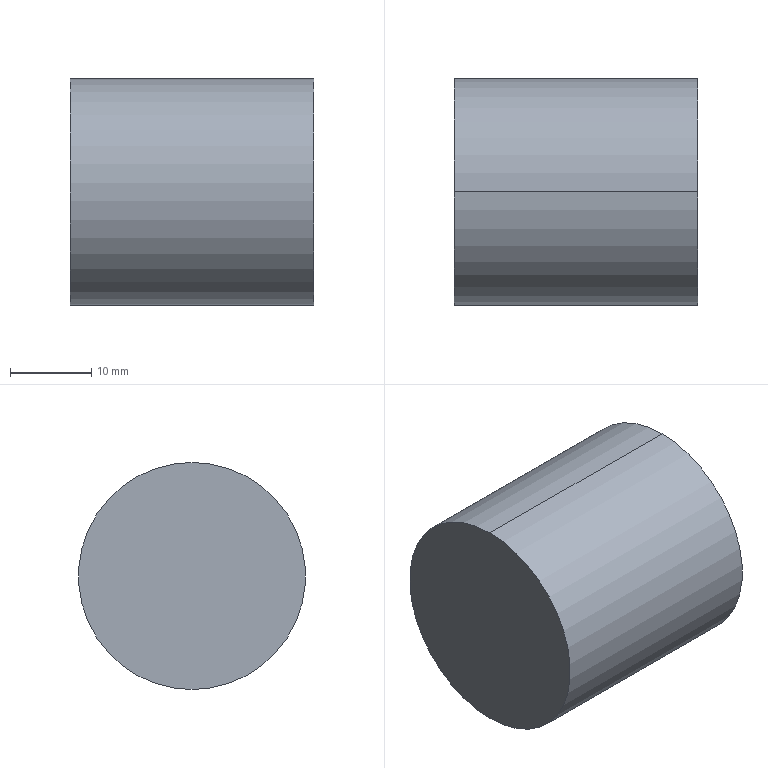Part | SolidWorks | features BaseBody 1 | 1 solid | 4 faces | box 30 x 28 x 28 mm | volume 18473 mm3 | cylinder 2 | plane 2 | commonest cylinder face diameters 28 x2
STEP:
#1=CARTESIAN_POINT('',(104.,23.,-152.));
#2=VERTEX_POINT('',#1);
#3=CARTESIAN_POINT('',(104.,23.,-124.));
#4=VERTEX_POINT('',#3);
#5=CARTESIAN_POINT('',(104.,23.,-138.));
#6=DIRECTION('',(1.,0.,0.));
#7=DIRECTION('',(0.,0.,-1.));
#8=AXIS2_PLACEMENT_3D('',#5,#6,#7);
#9=CIRCLE('',#8,14.);
#10=EDGE_CURVE('',#2,#4,#9,.T.);
#11=ORIENTED_EDGE('',*,*,#10,.T.);
#12=CARTESIAN_POINT('',(134.,23.,-124.));
#13=VERTEX_POINT('',#12);
#14=CARTESIAN_POINT('',(104.,23.,-124.));
#15=DIRECTION('',(1.,0.,0.));
#16=VECTOR('',#15,1000.);
#17=LINE('',#14,#16);
#18=EDGE_CURVE('',#4,#13,#17,.T.);
#19=ORIENTED_EDGE('',*,*,#18,.T.);
#20=CARTESIAN_POINT('',(134.,23.,-152.));
#21=VERTEX_POINT('',#20);
#22=CARTESIAN_POINT('',(134.,23.,-138.));
#23=DIRECTION('',(-1.,0.,0.));
#24=DIRECTION('',(0.,0.,-1.));
#25=AXIS2_PLACEMENT_3D('',#22,#23,#24);
#26=CIRCLE('',#25,14.);
#27=EDGE_CURVE('',#13,#21,#26,.T.);
#28=ORIENTED_EDGE('',*,*,#27,.T.);
#29=CARTESIAN_POINT('',(104.,23.,-152.));
#30=DIRECTION('',(1.,0.,0.));
#31=VECTOR('',#30,1000.);
#32=LINE('',#29,#31);
#33=EDGE_CURVE('',#2,#21,#32,.T.);
#34=ORIENTED_EDGE('',*,*,#33,.F.);
#35=EDGE_LOOP('',(#11,#19,#28,#34));
#36=FACE_OUTER_BOUND('',#35,.T.);
#37=CARTESIAN_POINT('',(104.,23.,-138.));
#38=DIRECTION('',(1.,0.,0.));
#39=DIRECTION('',(0.,0.,-1.));
#40=AXIS2_PLACEMENT_3D('',#37,#38,#39);
#41=CYLINDRICAL_SURFACE('',#40,14.);
#42=ADVANCED_FACE('',(#36),#41,.T.);
#43=ORIENTED_EDGE('',*,*,#18,.F.);
#44=CARTESIAN_POINT('',(104.,23.,-138.));
#45=DIRECTION('',(1.,0.,0.));
#46=DIRECTION('',(0.,0.,-1.));
#47=AXIS2_PLACEMENT_3D('',#44,#45,#46);
#48=CIRCLE('',#47,14.);
#49=EDGE_CURVE('',#4,#2,#48,.T.);
#50=ORIENTED_EDGE('',*,*,#49,.T.);
#51=ORIENTED_EDGE('',*,*,#33,.T.);
#52=CARTESIAN_POINT('',(134.,23.,-138.));
#53=DIRECTION('',(-1.,0.,0.));
#54=DIRECTION('',(0.,0.,-1.));
#55=AXIS2_PLACEMENT_3D('',#52,#53,#54);
#56=CIRCLE('',#55,14.);
#57=EDGE_CURVE('',#21,#13,#56,.T.);
#58=ORIENTED_EDGE('',*,*,#57,.T.);
#59=EDGE_LOOP('',(#43,#50,#51,#58));
#60=FACE_OUTER_BOUND('',#59,.T.);
#61=CARTESIAN_POINT('',(104.,23.,-138.));
#62=DIRECTION('',(1.,0.,0.));
#63=DIRECTION('',(0.,0.,-1.));
#64=AXIS2_PLACEMENT_3D('',#61,#62,#63);
#65=CYLINDRICAL_SURFACE('',#64,14.);
#66=ADVANCED_FACE('',(#60),#65,.T.);
#67=ORIENTED_EDGE('',*,*,#10,.F.);
#68=ORIENTED_EDGE('',*,*,#49,.F.);
#69=EDGE_LOOP('',(#67,#68));
#70=FACE_OUTER_BOUND('',#69,.T.);
#71=CARTESIAN_POINT('',(104.,23.,-138.));
#72=DIRECTION('',(1.,0.,0.));
#73=DIRECTION('',(0.,0.,-1.));
#74=AXIS2_PLACEMENT_3D('',#71,#72,#73);
#75=PLANE('',#74);
#76=ADVANCED_FACE('',(#70),#75,.F.);
#77=ORIENTED_EDGE('',*,*,#57,.F.);
#78=ORIENTED_EDGE('',*,*,#27,.F.);
#79=EDGE_LOOP('',(#77,#78));
#80=FACE_OUTER_BOUND('',#79,.T.);
#81=CARTESIAN_POINT('',(134.,23.,-138.));
#82=DIRECTION('',(1.,0.,0.));
#83=DIRECTION('',(0.,0.,-1.));
#84=AXIS2_PLACEMENT_3D('',#81,#82,#83);
#85=PLANE('',#84);
#86=ADVANCED_FACE('',(#80),#85,.T.);
#87=CLOSED_SHELL('',(#42,#66,#76,#86));
#88=MANIFOLD_SOLID_BREP('',#87);
#89=CARTESIAN_POINT('',(0.,0.,0.));
#90=DIRECTION('',(0.,0.,1.));
#91=DIRECTION('',(1.,0.,0.));
#92=AXIS2_PLACEMENT_3D('',#89,#90,#91);
#93=(LENGTH_UNIT()NAMED_UNIT(*)SI_UNIT(.MILLI.,.METRE.));
#94=UNCERTAINTY_MEASURE_WITH_UNIT(LENGTH_MEASURE(0.00001),#93,'','');
#95=(NAMED_UNIT(*)PLANE_ANGLE_UNIT()SI_UNIT($,.RADIAN.));
#96=(NAMED_UNIT(*)SI_UNIT($,.STERADIAN.)SOLID_ANGLE_UNIT());
#97=(GEOMETRIC_REPRESENTATION_CONTEXT(3)GLOBAL_UNCERTAINTY_ASSIGNED_CONTEXT((#94))GLOBAL_UNIT_ASSIGNED_CONTEXT((#93,#95,#96))REPRESENTATION_CONTEXT('',''));
#98=ADVANCED_BREP_SHAPE_REPRESENTATION('',(#88,#92),#97);